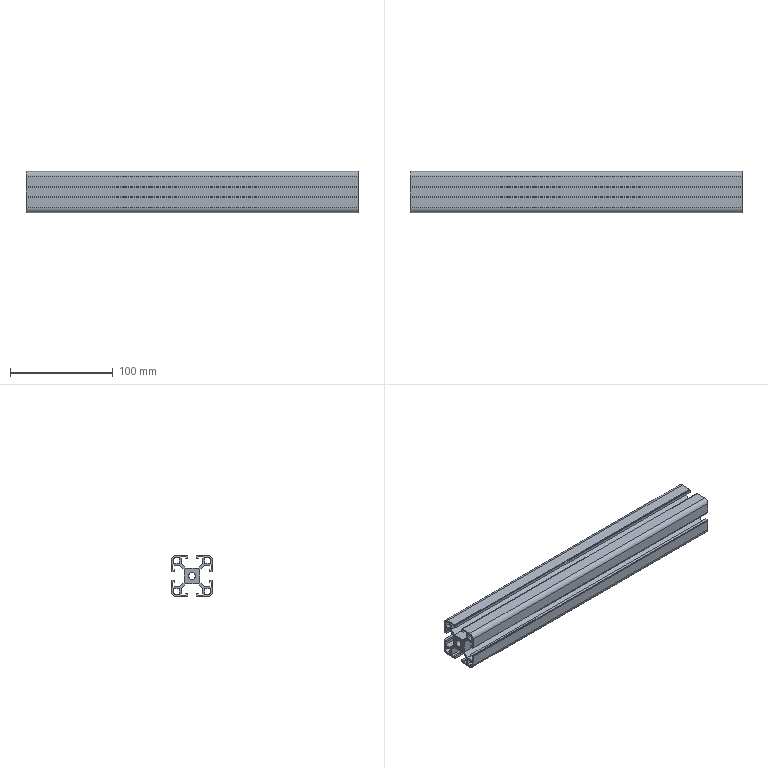Part | SolidWorks | features WeldMemberFeat 1, WeldmentFeature 1 | 1 solid | 104 faces | box 323 x 40 x 40 mm | volume 186224 mm3 | plane 94 | cylinder 10 | commonest cylinder face diameters 5 x4 9 x4 6.8 x2